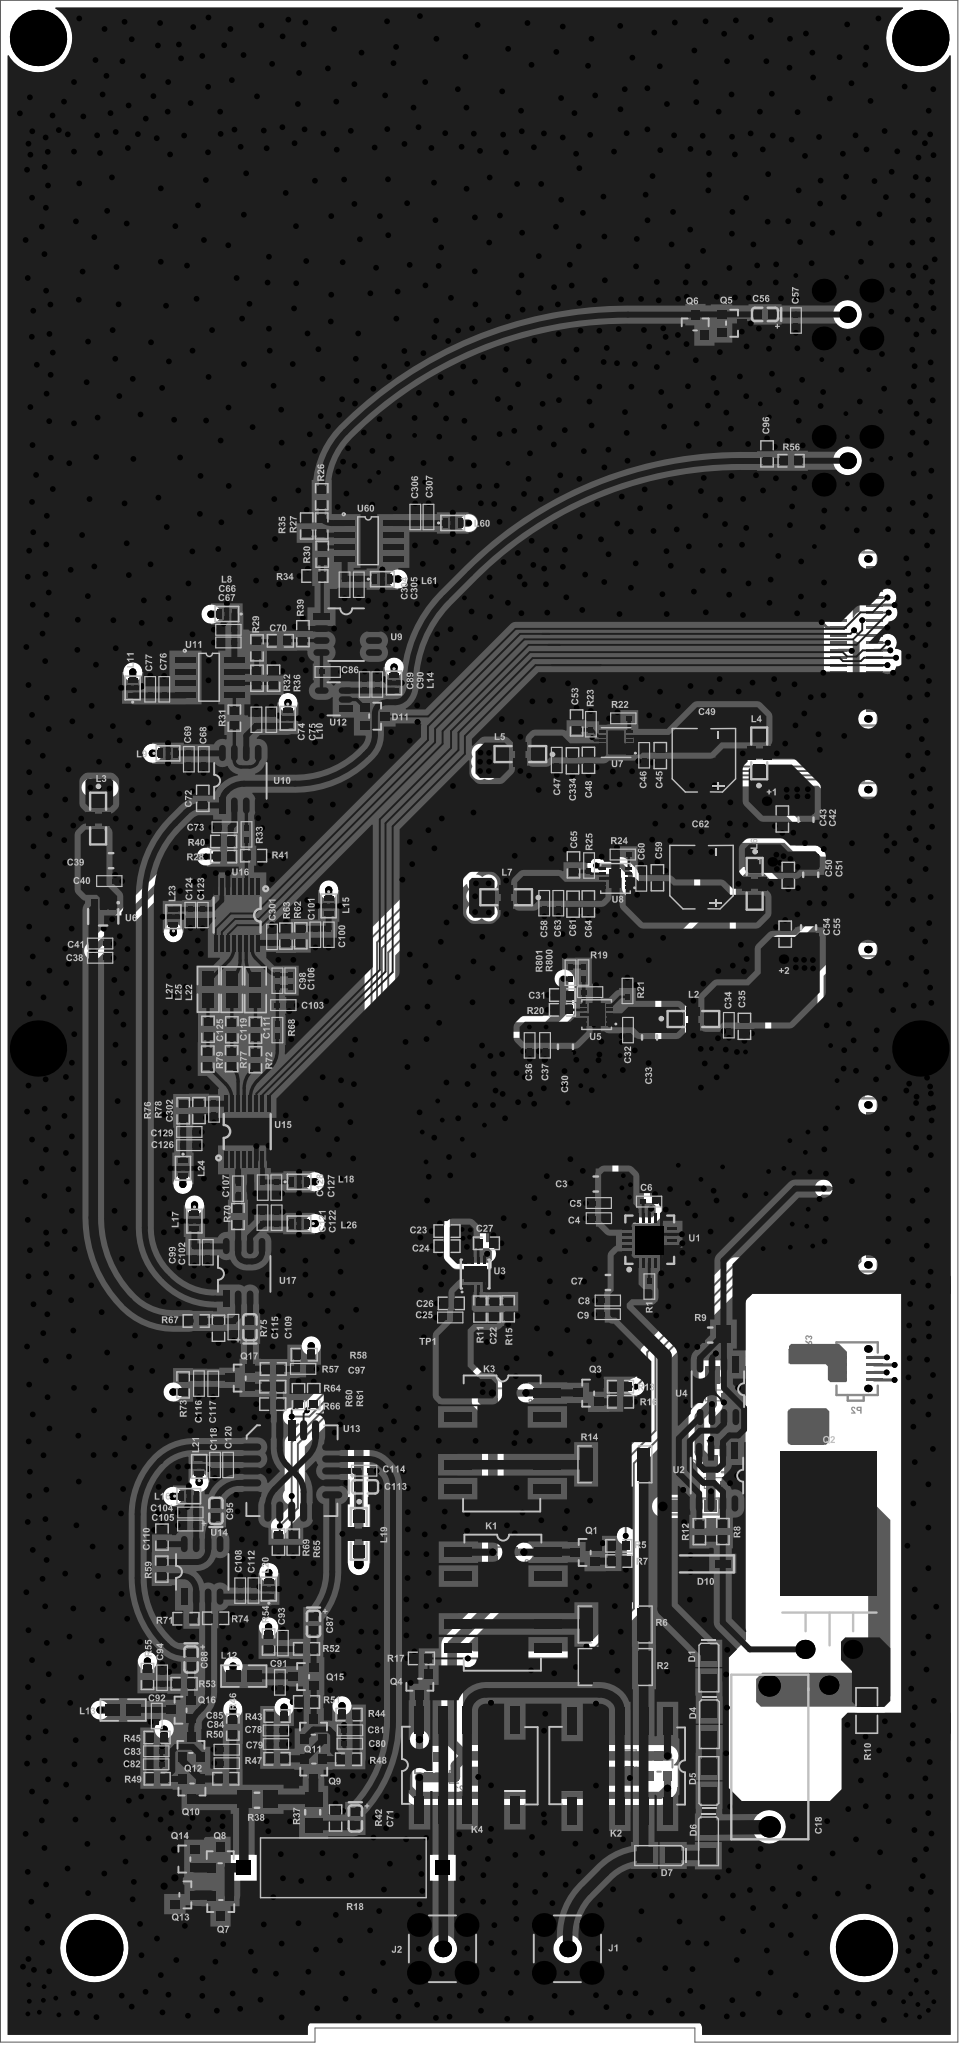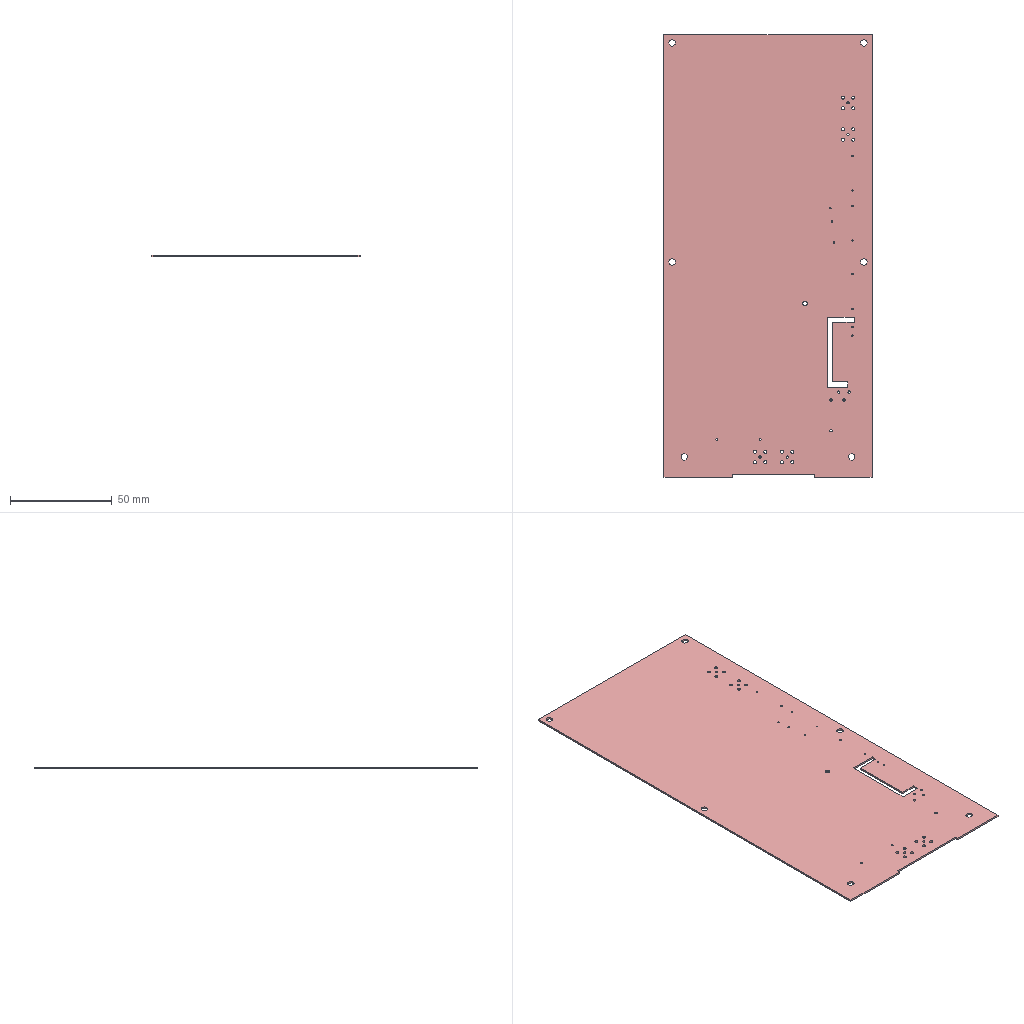Circuit board layout | Altium Designer | box 102 x 217 x 0.9 mm
Layer stack:
# Altium Designer layer stack of 10 (unit mm; dielectric type: 0 none, 1 core, 2 prepreg, 3 surface material)
index,name,kind,layer,copper_thickness_mm,dielectric_type,dielectric_thickness_mm,dielectric_material,dielectric_constant
0,TopPaste,other,,,,,,
1,TopOverlay,other,,,,,,
2,TopSolder,dielectric,,,3,0.0102,Solder Resist,3.5
3,TopLayer,copper,TopLayer,0.0356,,,,
4,Dielectric1,dielectric,,,1,0.32,FR-4,4.8
5,GND,copper,GND,0.036,,,,
6,Dielectric5,dielectric,,,2,0.127,,4.2
7,POWER,copper,POWER,0.036,,,,
8,Dielectric6,dielectric,,,1,0.254,,4.2
9,BottomLayer,copper,BottomLayer,0.0356,,,,
10,BottomSolder,dielectric,,,3,0.0102,Solder Resist,3.5
11,BottomOverlay,other,,,,,,
12,BottomPaste,other,,,,,,
# drill layer pairs: low layer,high layer
drill_pair,TopLayer,BottomLayer
Part placement:
Designator,Comment,Layer,Footprint,Center-X(mm),Center-Y(mm),Rotation
R801,4.7K 1%,TopLayer,0402,-29.527,-81.014,90
R800,523K 1%,TopLayer,0402,-28.13,-80.995,270
C14,0.1uF,BottomLayer,0402,-13.805,-125.946,360
C334,22uF 16V,TopLayer,0603,-29.305,-58.487,90
C61,22uF 16V,TopLayer,0603,-29.241,-73.72,90
U60,#NAME?,TopLayer,SOP8,-50.998,-35.128,0
L61,NFM18PC104R1C3D,TopLayer,FILTER-SMD_3P-L1.6-W0.8-L_NFM18CC223R1C3D,-49.556,-39.18,360
L60,NFM18PC104R1C3D,TopLayer,FILTER-SMD_3P-L1.6-W0.8-L_NFM18CC223R1C3D,-42.063,-33.21,360
C307,4.7uF 10V,TopLayer,0402,-44.636,-32.575,270
C306,0.1uF,TopLayer,0402,-46.063,-32.575,90
C305,4.7uF 10V,TopLayer,0402,-52.083,-39.777,90
C304,0.1uF,TopLayer,0402,-53.575,-39.776,270
C302,0.1uF,TopLayer,0402,-67.501,-95.543,90
C301,0.1uF,TopLayer,0402,-61.329,-77.204,90
R76,1K 1%,TopLayer,0603,-70.778,-95.686,270
L5,YFF31HC2A105MT000N,TopLayer,FILTER-SMD_4P-L3.2-W1.6-L_YFF31HC,-34.858,-57.773,180
C114,0.1uF,TopLayer,0402,-51.499,-133.947,180
C113,1UF 20V,TopLayer,0603钽电容,-51.409,-135.649,360
C107,0.1uF,TopLayer,0402,-64.922,-103.962,270
C106,1.2nF 1%,TopLayer,0402,-59.36,-81.852,270
C103,2.2nF 1%,TopLayer,0402,-60.11,-84.468,180
C99,0.1uF,TopLayer,0402,-69.584,-110.72,90
C98,2.2nF 1%,TopLayer,0402,-60.73,-81.864,270
C5,1uF 25V,TopLayer,0402,-26.505,-105.499,180
U17,AD603AR,TopLayer,SO8,-64.287,-112.852,90
U16,ADG658YRQZ,TopLayer,TSSOP-16_L5.0-W4.4-P0.65-LS6.4-TL,-65.038,-74.882,270
U15,ADG658YRQZ,TopLayer,TSSOP-16_L5.0-W4.4-P0.65-LS6.4-TL,-63.956,-97.902,90
U14,LMH6624MA(NS),TopLayer,SO8,-68.758,-144.526,90
U13,DG540DN PLCC20,TopLayer,QUAD20,-59.219,-133.963,0
U12,SN74AHC1G04DBVR,TopLayer,SOT25,-54.748,-51.975,180
U11,#NAME?,TopLayer,SOP8,-67.932,-49.632,360
U10,AD603AR,TopLayer,SO8,-64.694,-60.452,90
U9,MASWSS0157TR,TopLayer,SO8,-53.252,-45.073,360
U8,LT3045EDD#PBF,TopLayer,DFN-10_L3.0-W3.0-P0.50-BL-EP,-24.722,-70.984,90
U7,LT3094EDD#PBF,TopLayer,WDFN-12_L3.0-W3.0-P0.45-BL-EP,-24.657,-56.548,90
U6,#NAME?,TopLayer,TSOT-23-5_L2.9-W1.6-P0.95-LS2.8-BR,-79.298,-75.027,90
U5,GM12051ACPZ-R7,TopLayer,TDFN-10_L3.0-W3.0-P0.50-BL-EP,-26.728,-85.462,90
U4,TC4426COA(microchip),TopLayer,SO8,-13.805,-125.442,270
U3,TPL910A,TopLayer,DFN-8_L3.0-W3.0-P0.65-BL-EP2.3,-39.677,-113.103,0
U2,TC4426COA(microchip),TopLayer,SO8,-13.907,-134.626,270
U1,TPS7A4701RGWR,TopLayer,QFN-20,-21.128,-109.462,90
TP1,,TopLayer,TP1,-41.72,-119.927,0
R79,10R 1%,TopLayer,0603,-68.16,-90.187,270
R78,1.21K 1%,TopLayer,0603,-69.101,-95.661,270
R77,49.9R 1%,TopLayer,0603,-65.621,-90.149,270
R75,5.62K 1%,TopLayer,0603,-67.018,-118.792,90
R74,4.75K 1%,TopLayer,0603,-67.321,-149.619,180
R73,20R 1%,TopLayer,0603,-70.79,-124.82,270
R72,0R,TopLayer,0603,-63.08,-90.263,90
R71,118R 1%,TopLayer,0603,-70.482,-149.67,360
R70,10R 1%,TopLayer,0603,-64.948,-106.917,90
R69,20K 1%,TopLayer,0603,-60.63,-141.526,90
R68,0R,TopLayer,0402,-60.757,-87.11,90
R67,22.1K 1%,TopLayer,0603,-69.397,-118.022,180
R66,1K 1%,TopLayer,0603,-61.236,-126.861,360
R65,20K 1%,TopLayer,0603,-59.055,-141.526,270
R64,100R 1%,TopLayer,0603,-61.236,-125.007,360
R63,1.21K 1%,TopLayer,0603,-59.83,-77.119,270
R62,1K 1%,TopLayer,0603,-58.255,-77.086,90
R61,20K 1%,TopLayer,0603,-56.87,-126.057,90
R60,20K 1%,TopLayer,0603,-58.496,-126.065,270
R59,1K 1%,TopLayer,0603,-73.064,-144.396,90
R58,20R 1%,TopLayer,0603,-57.891,-121.603,180
R57,301R 1%,TopLayer,0603,-61.185,-123.127,360
R56,100R 1%,TopLayer,0603,-6.019,-26.598,360
R55,49.9R 1%,TopLayer,0603,-74.588,-155.807,270
R54,49.9R 1%,TopLayer,0603,-61.684,-152.142,90
R53,1K 1%,TopLayer,0603,-70.685,-156.578,360
R52,1K 1%,TopLayer,0603,-57.637,-152.87,180
R51,4.75K 1%,TopLayer,0603,-57.637,-158.521,180
R50,3.32K 1%,TopLayer,0603,-66.24,-166.675,360
R49,3.32K 1%,TopLayer,0603,-73.552,-166.675,360
R48,3.32K 1%,TopLayer,0603,-53.167,-164.605,180
R47,3.32K 1%,TopLayer,0603,-60.787,-164.554,180
R46,1.21K 1%,TopLayer,0603,-65.494,-161.193,270
R45,1.21K 1%,TopLayer,0603,-73.563,-162.294,180
R44,1.21K 1%,TopLayer,0603,-53.108,-159.855,360
R43,1.21K 1%,TopLayer,0603,-60.779,-160.008,360
R42,10R 1%,TopLayer,0603,-54.547,-170.845,270
R41,10K 1%,TopLayer,0603,-63.276,-68.568,180
R40,5.62K 1%,TopLayer,0603,-66.468,-67.069,360
R39,1.21K 1%,TopLayer,0603,-58.027,-44.98,90
R38,909R 1%,TopLayer,1206,-62.904,-168.859,270
R37,90.9R 1%,TopLayer,1206,-56.884,-170.244,180
R36,100R 1%,TopLayer,0603,-61.151,-49.704,90
R35,681R 1%,TopLayer,0603,-57.62,-33.532,90
R34,1K 1%,TopLayer,0603,-56.748,-38.85,180
R33,0R,TopLayer,0402,-64.047,-66.307,90
R32,681R 1%,TopLayer,0603,-62.916,-49.712,270
R31,100R 1%,TopLayer,0603,-65.329,-53.954,270
R30,100R 1%,TopLayer,0603,-55.969,-36.53,270
R29,10R 1%,TopLayer,0603,-62.916,-46.486,270
R28,22.1K 1%,TopLayer,0603,-66.468,-68.669,360
R27,681R 1%,TopLayer,0603,-56.02,-33.532,270
R26,47R 1%,TopLayer,0603,-56.02,-30.426,90
R25,49.9K 1%,TopLayer,0402,-27.548,-69.617,90
R24,0R,TopLayer,0402,-23.946,-68.466,180
R23,49.9K 1%,TopLayer,0402,-27.356,-54.6,90
R22,0R,TopLayer,0402,-23.889,-53.988,180
R21,0R,TopLayer,0402,-23.457,-82.944,90
R20,121K,TopLayer,0603,-30.379,-84.956,180
R19,13.3K  1%,TopLayer,0402,-27.43,-83.063,360
R18,51R 5W,TopLayer,5W,-53.717,-176.137,180
R17,10K 1%,TopLayer,0603,-45.4,-153.886,360
R16,10K 1%,TopLayer,0603,-24.19,-126.607,360
R15,10K 1%,TopLayer,0603,-36.156,-116.729,270
R14,82R 5% 3W,TopLayer,2512,-24.785,-133.262,360
R13,2.21K 1%,TopLayer,0603,-24.193,-125.007,360
R12,1.5R,TopLayer,0603,-15.786,-140.414,90
R11,52.5K 1%,TopLayer,0603,-39.154,-116.754,270
R10,0.5R 1%,TopLayer,0805,2.044,-159.424,90
R9,1.15K 1%,TopLayer,1206,-14.618,-119.419,270
R8,1.5R,TopLayer,0603,-13.282,-140.401,90
R7,10K 1%,TopLayer,0603,-24.367,-143.536,360
R6,220R 5% 1W,TopLayer,2512,-24.76,-150.28,360
R5,2.21K 1%,TopLayer,0603,-24.367,-141.923,360
R4,1K 1W,BottomLayer,2512,-4.28,-133.559,270
R3,1K 1W,BottomLayer,2512,-4.28,-124.988,90
R2,470R 5% 1W,TopLayer,2512,-24.746,-154.801,180
R1,0R,TopLayer,0402,-21.128,-114.364,90
Q17,BFT92,TopLayer,SOT23,-64.719,-124.066,90
Q16,PMBT3904,TopLayer,SOT23,-71.019,-159.359,90
Q15,PMBT3904,TopLayer,SOT23,-57.963,-155.791,90
Q14,MMBZ5257BLT1G,TopLayer,SOT23,-70.614,-175.184,90
Q13,MMBZ5257BLT1G,TopLayer,SOT23,-70.589,-179.045,270
Q12,MMBD7000LT1,TopLayer,SOT23,-69.927,-163.335,0
Q11,MMBD7000LT1,TopLayer,SOT23,-56.871,-161.392,360
Q10,MMBD7000LT1,TopLayer,SOT23,-69.876,-167.78,180
Q9,MMBD7000LT1,TopLayer,SOT23,-56.897,-165.659,180
Q8,MMBD7000LT1,TopLayer,SOT23,-66.804,-175.057,360
Q7,MMBD7000LT1,TopLayer,SOT23,-66.804,-180.163,180
Q6,MMBD914LT1G,TopLayer,SOT23,-16.206,-12.151,360
Q5,MMBD914LT1G,TopLayer,SOT23,-12.345,-12.011,270
Q4,2N7002-7-F,TopLayer,SOT23,-45.593,-156.642,180
Q3,PMBT3904,TopLayer,SOT23,-27.597,-125.666,90
Q2,STP10NK80Z,TopLayer,TO220,-1.994,-148.125,90
Q1,PMBT3904,TopLayer,SOT23,-27.966,-142.596,90
P9,RF connector straight jack,BottomLayer,DIP-P,0,-26.598,180
L27,3.9UH 5%,TopLayer,0805,-68.11,-82.779,90
L26,NFM18PC104R1C3D,TopLayer,FILTER-SMD_3P-L1.6-W0.8-L_NFM18CC223R1C3D,-58.446,-107.671,180
L25,10UH 5%,TopLayer,0805,-65.595,-82.804,90
L24,NFM18PC104R1C3D,TopLayer,FILTER-SMD_3P-L1.6-W0.8-L_NFM18CC223R1C3D,-70.803,-101.804,270
L23,NFM18PC104R1C3D,TopLayer,FILTER-SMD_3P-L1.6-W0.8-L_NFM18CC223R1C3D,-71.819,-75.058,90
L22,18UH 5%,TopLayer,0805,-63.08,-82.829,90
L21,NFM18PC104R1C3D,TopLayer,FILTER-SMD_3P-L1.6-W0.8-L_NFM18CC223R1C3D,-69.076,-133.478,90
L20,NFM18PC104R1C3D,TopLayer,FILTER-SMD_3P-L1.6-W0.8-L_NFM18CC223R1C3D,-61.659,-146.508,90
L19,YFF31HC2A105MT000N,TopLayer,FILTER-SMD_4P-L3.2-W1.6-L_YFF31HC,-52.071,-140.649,270
L18,NFM18PC104R1C3D,TopLayer,FILTER-SMD_3P-L1.6-W0.8-L_NFM18CC223R1C3D,-58.421,-103.239,360
L17,NFM18PC104R1C3D,TopLayer,FILTER-SMD_3P-L1.6-W0.8-L_NFM18CC223R1C3D,-69.584,-107.417,270
L16,NFM18PC104R1C3D,TopLayer,FILTER-SMD_3P-L1.6-W0.8-L_NFM18CC223R1C3D,-70.181,-136.64,360
L15,NFM18PC104R1C3D,TopLayer,FILTER-SMD_3P-L1.6-W0.8-L_NFM18CC223R1C3D,-55.284,-73.914,270
L14,NFM18PC104R1C3D,TopLayer,FILTER-SMD_3P-L1.6-W0.8-L_NFM18CC223R1C3D,-48.324,-50.216,270
L13,0.39UH 10%,TopLayer,0805,-77.178,-159.373,360
L12,0.39UH 10%,TopLayer,0805,-64.326,-155.766,360
L11,NFM18PC104R1C3D,TopLayer,FILTER-SMD_3P-L1.6-W0.8-L_NFM18CC223R1C3D,-76.162,-50.737,90
L10,NFM18PC104R1C3D,TopLayer,FILTER-SMD_3P-L1.6-W0.8-L_NFM18CC223R1C3D,-59.641,-53.975,270
L9,NFM18PC104R1C3D,TopLayer,FILTER-SMD_3P-L1.6-W0.8-L_NFM18CC223R1C3D,-72.391,-57.697,360
L8,NFM18PC104R1C3D,TopLayer,FILTER-SMD_3P-L1.6-W0.8-L_NFM18CC223R1C3D,-66.129,-42.888,180
L7,YFF31HC2A105MT000N,TopLayer,FILTER-SMD_4P-L3.2-W1.6-L_YFF31HC,-36.369,-72.987,180
L6,YFF31HC2A105MT000N,TopLayer,FILTER-SMD_4P-L3.2-W1.6-L_YFF31HC,-9.894,-71.561,270
L4,YFF31HC2A105MT000N,TopLayer,FILTER-SMD_4P-L3.2-W1.6-L_YFF31HC,-9.411,-57.701,90
L3,YFF31HC2A105MT000N,TopLayer,FILTER-SMD_4P-L3.2-W1.6-L_YFF31HC,-79.845,-64.627,270
L2,YFF31HC2A105MT000N,TopLayer,FILTER-SMD_4P-L3.2-W1.6-L_YFF31HC,-16.422,-85.931,360
L1,YFF31HC2A105MT000N,BottomLayer,FILTER-SMD_4P-L3.2-W1.6-L_YFF31HC,-16.451,-137.732,360
K4,TQ2SS-5V(ATQ209SS)SMD10,TopLayer,K,-40.525,-165.205,90
K3,TQ2SS-5V(ATQ209SS)SMD10,TopLayer,K,-36.757,-130.763,360
K2,TQ2SS-5V(ATQ209SS)SMD10,TopLayer,K,-24.261,-165.364,270
K1,TQ2SS-5V(ATQ209SS)SMD10,TopLayer,K,-36.681,-147.679,360
D11,MMBZ5231B,TopLayer,SOT23,-50.369,-53.772,270
D10,MMSZ5248B,TopLayer,1206D,-15.012,-143.799,180
D9,MMBD914LT1G,BottomLayer,SOT23,-44.628,-165.405,360
D8,MMBD914LT1G,BottomLayer,SOT23,-36.729,-126.645,270
D7,ES1D SMA,TopLayer,1606D,-20.097,-174.826,180
D6,DFLU1400-7,TopLayer,1606D,-14.83,-173.336,270
D5,3SMAJ5929B,TopLayer,1606D,-14.756,-166.898,90
D4,ES1D SMA,TopLayer,1606D,-14.735,-160.89,270
D3,MMBD914LT1G,BottomLayer,SOT23,-20.117,-165.329,180
D2,MMBD914LT1G,BottomLayer,SOT23,-36.729,-143.507,270
D1,ES1D SMA,TopLayer,1606D,-14.786,-154.87,270
C129,4.7uF 10V,TopLayer,0402,-70.129,-97.943,180
C128,0.1uF,TopLayer,0402,-62.319,-103.848,90
C127,4.7uF 10V,TopLayer,0402,-60.872,-103.848,90
C126,0.1uF,TopLayer,0402,-70.129,-99.353,180
C125,56pF 1%,TopLayer,0603,-68.135,-87.02,270
C124,0.1uF,TopLayer,0402,-70.003,-74.88,270
C123,4.7uF 10V,TopLayer,0402,-68.708,-74.88,90
C122,4.7uF 10V,TopLayer,0402,-60.81,-107.049,270
C121,0.1uF,TopLayer,0402,-62.319,-107.036,270
C120,4.7uF 10V,TopLayer,0402,-66.009,-133.325,90
C119,100pF 1%,TopLayer,0603,-65.596,-87.076,270
C118,0.1uF,TopLayer,0402,-67.399,-133.327,90
C117,4.7uF 10V,TopLayer,0402,-67.59,-124.702,90
C116,0.1uF,TopLayer,0402,-69.114,-124.676,90
C115,0.1uF,TopLayer,0402,-65.418,-118.674,270
C112,4.7uF 10V,TopLayer,0402,-63.285,-146.673,270
C111,270pF 1%,TopLayer,0603,-63.08,-87.113,270
C110,0.1uF,TopLayer,0603,-73.038,-140.991,270
C109,2.2UF 10V,TopLayer,0603钽电容,-63.666,-118.693,90
C108,0.1uF,TopLayer,0402,-64.695,-146.685,270
C105,0.1uF,TopLayer,0402,-70.028,-139.751,360
C104,4.7uF 10V,TopLayer,0402,-70.016,-138.367,360
C102,4.7uF 10V,TopLayer,0402,-68.175,-110.72,90
C101,0.1uF,TopLayer,0402,-56.693,-76.975,270
C100,4.7uF 10V,TopLayer,0402,-55.284,-76.975,90
C97,0.1uF,TopLayer,0402,-58.001,-123.127,180
C96,NC,TopLayer,0603,-8.575,-25.871,90
C95,10uF 10V,TopLayer,0603钽电容,-67.298,-138.2,90
C94,0.1uF,TopLayer,0402,-73.013,-155.943,270
C93,0.1uF,TopLayer,0402,-60.148,-152.26,270
C92,0.1uF,TopLayer,0402,-73.584,-160.007,270
C91,0.1uF,TopLayer,0402,-60.465,-156.439,270
C90,0.1uF,TopLayer,0402,-50.115,-50.38,90
C89,4.7uF 10V,TopLayer,0402,-51.436,-50.38,270
C88,1UF 20V,TopLayer,0603钽电容,-69.939,-154.002,270
C87,1UF 20V,TopLayer,0603钽电容,-56.897,-150.202,270
C86,10pF,TopLayer,0402,-55.385,-49.035,360
C85,4.7uF 10V,TopLayer,0402,-66.142,-163.576,360
C84,0.1uF,TopLayer,0402,-66.142,-165.011,360
C83,0.1uF,TopLayer,0402,-73.648,-163.742,360
C82,4.7uF 10V,TopLayer,0402,-73.661,-165.152,180
C81,4.7uF 10V,TopLayer,0402,-53.011,-161.519,360
C80,0.1uF,TopLayer,0402,-53.023,-162.954,180
C79,0.1uF,TopLayer,0402,-60.897,-163.005,180
C78,4.7uF 10V,TopLayer,0402,-60.897,-161.557,180
C77,4.7uF 10V,TopLayer,0402,-74.283,-50.889,270
C76,0.1uF,TopLayer,0402,-72.81,-50.889,90
C75,4.7uF 10V,TopLayer,0402,-61.38,-54.126,270
C74,0.1uF,TopLayer,0402,-62.989,-54.126,90
C73,0.1uF,TopLayer,0402,-66.358,-65.571,180
C72,NC,TopLayer,0603,-68.695,-62.481,90
C71,1UF 20V,TopLayer,0603钽电容,-52.439,-170.893,270
C70,10nF,TopLayer,0603,-60.431,-45.733,180
C69,0.1uF,TopLayer,0402,-70.164,-58.321,270
C68,4.7uF 10V,TopLayer,0402,-68.606,-58.321,90
C67,0.1uF,TopLayer,0402,-65.964,-45.923,180
C66,4.7uF 10V,TopLayer,0402,-65.964,-44.554,360
C65,22uF 16V,TopLayer,0603,-29.198,-69.55,270
C64,22uF 16V,TopLayer,0603,-27.616,-73.694,90
C63,10nF,TopLayer,0402,-30.804,-73.622,270
C62,220UF10V (D6.3*7.7mm),TopLayer,CAP-SMD_BD6.3-L6.6-W6.6-FD,-15.558,-70.851,90
C60,0.1uF,TopLayer,0402,-21.99,-70.993,90
C59,22uF 16V,TopLayer,0603,-20.257,-70.921,270
C58,0.1uF,TopLayer,0402,-32.303,-73.622,270
C57,10pF,TopLayer,0402,-5.512,-11.693,90
C56,2.2UF 10V,TopLayer,0603钽电容,-8.79,-11.046,180
C55,47uF 25V,TopLayer,1206,-4.052,-76.213,180
C54,0.1uF,TopLayer,0603,-6.643,-76.908,90
C53,22uF 16V,TopLayer,0603,-28.868,-54.462,90
C51,47uF 25V,TopLayer,1206,-4.026,-70.589,0
C50,0.1uF,TopLayer,0603,-6.312,-70.659,90
C49,220UF10V (D6.3*7.7mm),TopLayer,CAP-SMD_BD6.3-L6.6-W6.6-FD,-15.304,-58.43,90
C48,22uF 16V,TopLayer,0603,-27.604,-58.436,90
C47,0.1uF,TopLayer,0402,-30.97,-58.408,270
C46,0.1uF,TopLayer,0402,-21.654,-57.9,270
C45,22uF 16V,TopLayer,0603,-19.952,-57.934,90
C43,0.1uF,TopLayer,0603,-6.947,-64.673,270
C42,47uF 25V,TopLayer,1206,-4.534,-64.732,0
C41,0.1uF,TopLayer,0402,-79.628,-77.923,180
C40,0.1uF,TopLayer,0402,-78.652,-71.286,180
C39,47uF 25V,TopLayer,1206,-78.474,-69.203,90
C38,4.7uF 10V,TopLayer,0402,-79.628,-79.435,180
C37,0.1uF,TopLayer,0402,-32.218,-88.728,270
C36,0.1uF,TopLayer,0402,-33.859,-88.735,270
C35,4.7uF 25V,TopLayer,0603,-10.986,-86.709,270
C34,0.1uF,TopLayer,0402,-12.633,-86.591,270
C33,47uF 25V,TopLayer,1206,-21.197,-87.872,360
C32,0.1uF,TopLayer,0402,-23.381,-87.11,270
C31,4.7uF 25V,TopLayer,0603,-30.354,-83.381,180
C30,47uF 25V,TopLayer,1206,-30.156,-88.867,360
C29,47uF 25V,BottomLayer,1206,-13.17,-133.185,270
C28,0.1uF,BottomLayer,0402,-13.907,-135.258,360
C27,0.1uF,TopLayer,0603,-38.478,-109.767,360
C26,22uF 16V,TopLayer,0603,-42.218,-116.153,180
C25,0.1uF,TopLayer,0402,-42.329,-117.665,180
C24,0.1uF,TopLayer,0603,-42.675,-110.071,180
C23,22uF 16V,TopLayer,0603,-42.675,-108.471,360
C22,10nF,TopLayer,0603,-37.655,-116.754,270
C21,10uF 10V,BottomLayer,0603,-41.025,-166.485,180
C20,10uF 10V,BottomLayer,0603,-37.063,-123.889,180
C18,0.1uF 5% 630V,TopLayer,AXIAL0.59,-8.355,-164.298,270
C17,10uF 10V,BottomLayer,0603,-23.178,-164.995,90
C16,10uF 10V,BottomLayer,0603,-37.038,-140.577,180
C15,47uF 25V,BottomLayer,1206,-13.043,-123.762,270
C9,1uF 25V,TopLayer,0402,-25.552,-117.31,180
C8,0.1uF,TopLayer,0402,-25.54,-115.863,180
C7,47uF 25V,TopLayer,1206,-25.515,-113.831,270
C6,1uF 25V,TopLayer,0402,-21.143,-105.322,360
C4,0.1uF,TopLayer,0402,-26.492,-107.112,180
C3,47uF 25V,TopLayer,1206,-26.81,-103.366,270
1,,TopLayer,DIP-1,-8.014,-69.228,90
+2,,TopLayer,DIP-1,-6.82,-79.566,0
+1,,TopLayer,DIP-1,-8.624,-62.777,0
P5,Header 20X2,BottomLayer,N0.8mm/40Pin-Plug,0.9204,-70.049,270
P6,RF connector straight jack,BottomLayer,DIP-P,0,-11.058,180
J1,RF connector right-angle socket,TopLayer,DIP-P,-29.82,-184.76,90
J2,RF connector right-angle socket,TopLayer,DIP-P,-43.129,-184.76,90
P1,Header 20X2,BottomLayer,N0.8mm/40Pin-Plug,0.9204,-103.561,270
P2,Header 4X2,BottomLayer,N0.8mm/8Pin-SOCKET,0.9204,-123.093,270
P4,Header 20X2,BottomLayer,N0.8mm/40Pin-Plug,0.9204,-45.535,270
Pad and via stacks:
# Altium Designer via and pad stacks of 10 (unit mm). Each distinct definition once, with the count of objects using it.
# via: kind,start_layer,end_layer,hole_mm,diameter_mm,mode(0 simple;1 top-mid-bottom;2 full stack),diameter_per_layer,count,example_net
# pad: kind,layer,hole_mm,hole_type(0 round;1 square;2 slot),plating,top_size,top_shape(1 round;2 rect;3 octagon;9 rounded rect),mid_size,bottom_size,mode,footprint,size_per_layer,count,example
pad,MultiLayer,0.68,0,plated,0.8x0.8,1,0.8x0.8,0.8x0.8,0,N0.8mm/40Pin-Plug,,6,P4.0
pad,MultiLayer,3.2,0,plated,6x6,1,6x6,6x6,0,,,6,2
pad,MultiLayer,0.68,0,plated,0.8x0.8,1,0.8x0.8,0.8x0.8,0,N0.8mm/8Pin-SOCKET,,2,P2.0
pad,MultiLayer,1.524,0,plated,2.54x2.54,1,2.54x2.54,2.54x2.54,0,DIP-P,,16,J1.1
pad,MultiLayer,1.143,0,plated,1.778x1.778,1,1.778x1.778,1.778x1.778,0,DIP-P,,4,J1.5
pad,MultiLayer,0.635,0,plated,1.016x1.016,1,1.016x1.016,1.016x1.016,0,DIP-1,,3,1.1
pad,MultiLayer,2.159,0,plated,3.048x3.048,2,3.048x3.048,3.048x3.048,0,QFN-20,,1,U1.21
pad,MultiLayer,1.143,0,plated,2.286x2.286,1,2.286x2.286,2.286x2.286,0,AXIAL0.59,,2,C18.2
pad,MultiLayer,1.143,0,plated,2.032x2.032,1,2.032x2.032,2.032x2.032,0,TO220,,3,Q2.3
pad,MultiLayer,1,0,plated,1.5x1.5,2,1.5x1.5,1.5x1.5,0,5W,,2,R18.2
pad,BottomLayer,0,0,plated,0.3x1.8,2,0.3x1.8,0.3x1.8,0,N0.8mm/40Pin-Plug,,120,P4.40
pad,BottomLayer,0,0,plated,0.3x1.8,2,0.3x1.8,0.3x1.8,0,N0.8mm/8Pin-SOCKET,,8,P2.2
pad,BottomLayer,0,0,plated,1.829x1.575,2,1.829x1.575,1.829x1.575,0,1206,,4,C15.2
pad,BottomLayer,0,0,plated,0.635x0.508,2,0.635x0.508,0.635x0.508,0,0402,,4,C14.2
pad,BottomLayer,0,0,plated,1.016x0.889,2,1.016x0.889,1.016x0.889,0,SOT23,,12,D3.1
pad,BottomLayer,0,0,plated,0.8065x0.864,2,0.8065x0.864,0.8065x0.864,0,0603,,8,C17.1
pad,BottomLayer,0,0,plated,1.4x0.9,2,1.4x0.9,1.4x0.9,0,FILTER-SMD_4P-L3.2-W1.6-L_YFF31HC,,2,L1.4
pad,BottomLayer,0,0,plated,1.3x1.2,2,1.3x1.2,1.3x1.2,0,FILTER-SMD_4P-L3.2-W1.6-L_YFF31HC,,2,L1.3
pad,BottomLayer,0,0,plated,1.282x3.456,2,1.282x3.456,1.282x3.456,0,2512,,4,R4.1
pad,TopLayer,0,0,plated,0.3048x1.016,2,0.3048x1.016,0.3048x1.016,0,QFN-20,,20,U1.2
pad,TopLayer,0,0,plated,1.524x1.27,2,1.524x1.27,1.524x1.27,0,0805,,12,L12.1
pad,TopLayer,0,0,plated,1.635x1.6,2,1.635x1.6,1.635x1.6,0,1606D,,10,D7.1
pad,TopLayer,0,0,plated,15.367x10.287,2,15.367x10.287,15.367x10.287,0,TO220,,1,Q2.4
pad,TopLayer,0,0,plated,1.829x1.575,2,1.829x1.575,1.829x1.575,0,1206,,22,R9.1
pad,TopLayer,0,0,plated,0.7112x1.727,1,0.7112x1.727,0.7112x1.727,0,SO8,,42,U4.8
pad,TopLayer,0,0,plated,0.7112x1.727,2,0.7112x1.727,0.7112x1.727,0,SO8,,6,U4.1
pad,TopLayer,0,0,plated,1.626x0.8128,2,1.626x0.8128,1.626x0.8128,0,1206D,,2,D10.1
pad,TopLayer,0,0,plated,0.8065x0.864,2,0.8065x0.864,0.8065x0.864,0,0603,,170,R12.1
pad,TopLayer,0,0,plated,1.016x0.889,2,1.016x0.889,1.016x0.889,0,SOT23,,51,Q3.2
pad,TopLayer,0,0,plated,1.282x3.456,2,1.282x3.456,1.282x3.456,0,2512,,6,R14.2
pad,TopLayer,0,0,plated,2.921x1.016,2,2.921x1.016,2.921x1.016,0,K,,40,K2.1
pad,TopLayer,0,0,plated,0.635x0.508,2,0.635x0.508,0.635x0.508,0,0402,,174,R1.2
pad,TopLayer,0,0,plated,2.159x2.159,1,2.159x2.159,2.159x2.159,0,TP1,,1,TP1.1
pad,TopLayer,0,0,plated,2.45x1.65,2,2.45x1.65,2.45x1.65,0,DFN-8_L3.0-W3.0-P0.65-BL-EP2.3,,1,U3.9
pad,TopLayer,0,0,plated,0.28x0.665,2,0.28x0.665,0.28x0.665,0,DFN-8_L3.0-W3.0-P0.65-BL-EP2.3,,8,U3.8
pad,TopLayer,0,0,plated,0.85x0.9,2,0.85x0.9,0.85x0.9,0,0603\u00EE\u00E3\u00B5\u00E7\u00C8\u00DD,,14,C71.2
pad,TopLayer,0,0,plated,0.5x0.4,2,0.5x0.4,0.5x0.4,0,FILTER-SMD_3P-L1.6-W0.8-L_NFM18CC223R1C3D,,32,L20.2
pad,TopLayer,0,0,plated,1x0.5,2,1x0.5,1x0.5,0,FILTER-SMD_3P-L1.6-W0.8-L_NFM18CC223R1C3D,,32,L20.3
pad,TopLayer,0,0,plated,1.4x0.9,2,1.4x0.9,1.4x0.9,0,FILTER-SMD_4P-L3.2-W1.6-L_YFF31HC,,14,L19.4
pad,TopLayer,0,0,plated,1.3x1.2,2,1.3x1.2,1.3x1.2,0,FILTER-SMD_4P-L3.2-W1.6-L_YFF31HC,,14,L19.3
pad,TopLayer,0,0,plated,0.762x2.159,1,0.762x2.159,0.762x2.159,0,QUAD20,,19,U13.10
pad,TopLayer,0,0,plated,0.762x2.159,2,0.762x2.159,0.762x2.159,0,QUAD20,,1,U13.1
pad,TopLayer,0,0,plated,1.803x0.4064,2,1.803x0.4064,1.803x0.4064,0,TSSOP-16_L5.0-W4.4-P0.65-LS6.4-TL,,32,U15.16
pad,TopLayer,0,0,plated,1.1x0.7,2,1.1x0.7,1.1x0.7,0,TSOT-23-5_L2.9-W1.6-P0.95-LS2.8-BR,,5,U6.5
pad,TopLayer,0,0,plated,0.6858x1.473,2,0.6858x1.473,0.6858x1.473,0,SOT25,,1,U12.1
pad,TopLayer,0,0,plated,0.6858x1.473,1,0.6858x1.473,0.6858x1.473,0,SOT25,,4,U12.2
pad,TopLayer,0,0,plated,2.159x0.635,2,2.159x0.635,2.159x0.635,0,SOP8,,16,U11.6
pad,TopLayer,0,0,plated,0.252x0.665,2,0.252x0.665,0.252x0.665,0,WDFN-12_L3.0-W3.0-P0.45-BL-EP,,12,U7.1
pad,TopLayer,0,0,plated,2.4x1.7,2,2.4x1.7,2.4x1.7,0,WDFN-12_L3.0-W3.0-P0.45-BL-EP,,1,U7.13
pad,TopLayer,0,0,plated,3.5x1.2,2,3.5x1.2,3.5x1.2,0,CAP-SMD_BD6.3-L6.6-W6.6-FD,,4,C49.1
pad,TopLayer,0,0,plated,2x1.2,2,2x1.2,2x1.2,0,DFN-10_L3.0-W3.0-P0.50-BL-EP,,1,U8.11
pad,TopLayer,0,0,plated,0.25x0.65,2,0.25x0.65,0.25x0.65,0,DFN-10_L3.0-W3.0-P0.50-BL-EP,,10,U8.10
pad,TopLayer,0,0,plated,0.28x0.665,2,0.28x0.665,0.28x0.665,0,TDFN-10_L3.0-W3.0-P0.50-BL-EP,,10,U5.1
pad,TopLayer,0,0,plated,2.4x1.7,2,2.4x1.7,2.4x1.7,0,TDFN-10_L3.0-W3.0-P0.50-BL-EP,,1,U5.11
via,TopLayer,BottomLayer,0.3048,0.6096,0,,2014,GND
via,TopLayer,BottomLayer,0.3048,0.508,0,,116,12.4V
via,TopLayer,BottomLayer,0.508,1.016,0,,2,H12V
via,TopLayer,BottomLayer,0.381,0.762,0,,38,NetD3_1
Copper pours:
name,layer,net,type(0 solid;1 hatched;2 none)
Bottom Layer-No Net,TopLayer,12.4V,0
Bottom Layer-No Net,TopLayer,A6V,0
-5.4V_L01_P000,TopLayer,-5.4V,0
NETC45_2_L01_P004,TopLayer,NetC45_2,0
A6V_L01_P008,TopLayer,A6V,0
NETC59_2_L01_P012,TopLayer,NetC59_2,0
NETC58_1_L01_P014,TopLayer,NetC58_1,0
12.4V_L01_P016,TopLayer,12.4V,0
NETC32_1_L01_P022,TopLayer,NetC32_1,0
A12V_L01_P024,TopLayer,A12V,0
NETC39_1_L01_P028,TopLayer,NetC39_1,0
H12V_L01_P042,TopLayer,H12V,0
H5V_L01_P044,TopLayer,H5V,0
NETQ2_3_L01_P054,TopLayer,NetQ2_3,0
+5V_L01_P056,TopLayer,+5V,0
+5V_L01_P060,TopLayer,+5V,0
-5V_L01_P062,TopLayer,-5V,0
NETC47_1_L01_P006,TopLayer,NetC47_1,0
GND_L01_P064,TopLayer,GND,0
Bottom Layer-No Net,BottomLayer,A6V,0
Bottom Layer-No Net,BottomLayer,12.4V,0
-5.4V_L04_P002,BottomLayer,-5.4V,0
A6V_L04_P010,BottomLayer,A6V,0
H5V_L04_P046,BottomLayer,H5V,0
HT_L04_P048,BottomLayer,HT,0
NETR3_1_L04_P050,BottomLayer,NetR3_1,0
GND_L04_P066,BottomLayer,GND,0
NETC18_1_L04_P052,BottomLayer,NetC18_1,0
Design rules, without the lines most boards share:
# Altium Designer design rules of 10 (exported by Altium Designer, unit mm)
# columns: name | kind | enabled | priority | scope1 | scope2 | descriptor | typed fields (field=value)
Clearance_2 | 0 | enabled | 2 | inpolygon | All | Clearance Constraint (Gap=6mil) (inpolygon),(All) | gap=0.1524
SilkToSilkClearance | 55 | enabled | 1 | All | All | Silk to Silk (Clearance=0mil) (All),(All) |
SilkscreenOverComponentPads | 54 | enabled | 1 | IsPad | All | Silk To Solder Mask (Clearance=0mil) (IsPad),(All) |
MinimumSolderMaskSliver | 53 | enabled | 1 | All | All | Minimum Solder Mask Sliver (Gap=0mil) (All),(All) |
HoleToHoleClearance | 52 | enabled | 1 | All | All | Hole To Hole Clearance (Gap=0mil) (All),(All) | gap=0
DiffPairsRouting | 51 | enabled | 1 | All | All | Differential Pairs Uncoupled Length using the Gap Constraints (Min=6mil) (Max=6mil) (Prefered=6mil)  and Width Constraints (Min=15mil) (Max=15mil) (Prefered=15mil) (All) |
Clearance | 0 | enabled | 4 | All | All | Clearance Constraint (Gap=6mil) (All),(All) | gap=0.1524
Testpoint | 43 | enabled | 1 | All | All | Fabrication Testpoint Style (Under Component=Yes) (All) |
TestPointUsage | 44 | enabled | 1 | All | All | Fabrication Testpoint Usage (Valid =One Required, Allow multiple per net=No) (All) |
SolderMaskExpansion | 13 | enabled | 1 | All | All | Solder Mask Expansion (Expansion =4mil) (All) | expansion=0.1016
PasteMaskExpansion | 14 | enabled | 1 | All | All | Paste Mask Expansion (Expansion =0mil) (All) | expansion=0
RoutingVias | 11 | enabled | 1 | All | All | Routing Via (MinHoleWidth=12mil) (MaxHoleWidth=20mil) (PreferredHoleWidth=12mil) (MinWidth=20mil) (MaxWidth=40mil) (PreferedWidth=20mil) (All) | via_min_hole=0.3048 via_max_hole=0.508 via_preferred_diameter=0.508 via_preferred_hole=0.3048
Width | 2 | enabled | 1 | All | All | Width Constraint (Min=8mil) (Max=200mil) (Preferred=10mil) (All) |
PolygonConnect | 20 | enabled | 1 | All | All | Polygon Connect Rule(Direct Connect )(Conductor Width=10mil) (Relief Angle=90 Angle) (Entries=4) (Air Gap Width=10mil) (All),(All) | connect_style(0=relief,1=direct,2=none)=1 relief_conductor_width=0.254 relief_entries=4
PlaneClearance | 12 | enabled | 1 | All | All | Power Plane Clearance (Clearance =6mil) (All) | clearance=0.1524
PlaneConnect | 6 | enabled | 1 | All | All | Power Plane Connect Rule(Direct Connect )(Expansion=20mil) (Conductor Width=10mil) (Air Gap=10mil) (Entries=4) (All) | relief_conductor_width=0.254 relief_entries=4 relief_expansion=0.508
Clearance_1 | 0 | disabled | 3 | (IsKeepOut) | All | Clearance Constraint (Gap=6mil) (Disabled)((IsKeepOut)),(All) | gap=0.1524
HoleSize | 42 | disabled | 1 | All | All | Hole Size Constraint (Min=1mil) (Max=500mil) (Disabled)(All) |
ComponentClearance | 24 | disabled | 1 | All | All | Component Clearance Constraint ( Horizontal Gap = 10mil, Vertical Gap = 10mil ) (Disabled)(All),(All)  | gap=0.254
Clearance_3 | 0 | enabled | 1 | ispad | ispad | Clearance Constraint (Gap=6mil) (ispad),(ispad) | gap=0.1524
Classes set for this board:
# Altium Designer classes of 10 (member kind: 0 net, 1 component, 2 from-to, 3 pad, 4 layer, 5 differential pair, 6 design channel, 7 polygon, 8 structure, 9 xSignal)
# columns: class name | member kind | superclass | members
All From-Tos | 0 | yes |